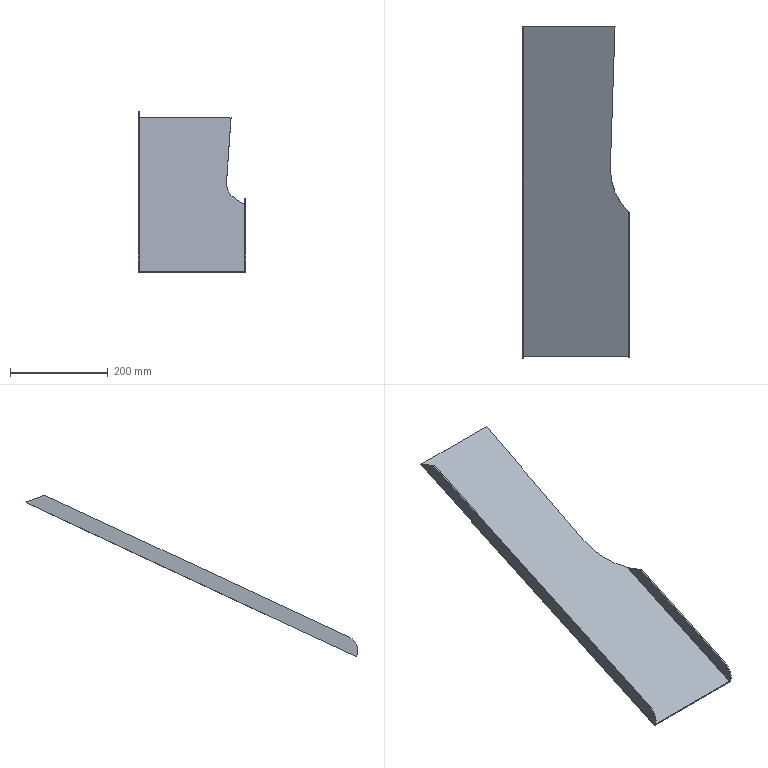Part | NX | features solid 2 | 1 solid | 15 faces | box 219.206 x 677.811 x 330.114 mm | volume 356857 mm3 | plane 12 | cylinder 2 | spline 1 | commonest cylinder face diameters 60 x2
STEP:
#1=CARTESIAN_POINT('',(-1052.794,-840.,-504.758));
#2=VERTEX_POINT('',#1);
#3=CARTESIAN_POINT('',(-1268.,-840.,-504.758));
#4=VERTEX_POINT('',#3);
#5=CARTESIAN_POINT('',(-476.248,-840.,-504.758));
#6=DIRECTION('',(1.,0.,0.));
#7=VECTOR('',#6,1000.);
#8=LINE('',#5,#7);
#9=EDGE_CURVE('',#2,#4,#8,.F.);
#10=ORIENTED_EDGE('',*,*,#9,.F.);
#11=CARTESIAN_POINT('',(-1052.794,-840.,-502.551));
#12=VERTEX_POINT('',#11);
#13=CARTESIAN_POINT('',(-1052.794,-840.,-720.));
#14=DIRECTION('',(0.,0.,-1.));
#15=VECTOR('',#14,1000.);
#16=LINE('',#13,#15);
#17=EDGE_CURVE('',#2,#12,#16,.F.);
#18=ORIENTED_EDGE('',*,*,#17,.T.);
#19=CARTESIAN_POINT('',(-1268.,-840.,-502.551));
#20=VERTEX_POINT('',#19);
#21=CARTESIAN_POINT('',(-476.248,-840.,-502.551));
#22=DIRECTION('',(1.,0.,0.));
#23=VECTOR('',#22,1000.);
#24=LINE('',#21,#23);
#25=EDGE_CURVE('',#12,#20,#24,.F.);
#26=ORIENTED_EDGE('',*,*,#25,.T.);
#27=CARTESIAN_POINT('',(-1268.,-840.,-720.));
#28=DIRECTION('',(0.,0.,1.));
#29=VECTOR('',#28,1000.);
#30=LINE('',#27,#29);
#31=EDGE_CURVE('',#20,#4,#30,.F.);
#32=ORIENTED_EDGE('',*,*,#31,.T.);
#33=EDGE_LOOP('',(#10,#18,#26,#32));
#34=FACE_BOUND('',#33,.T.);
#35=CARTESIAN_POINT('',(-476.248,-840.,-720.));
#36=DIRECTION('',(0.,1.,0.));
#37=DIRECTION('',(-1.,0.,0.));
#38=AXIS2_PLACEMENT_3D('',#35,#36,#37);
#39=PLANE('',#38);
#40=ADVANCED_FACE('',(#34),#39,.F.);
#41=ORIENTED_EDGE('',*,*,#25,.F.);
#42=CARTESIAN_POINT('',(-1052.794,-547.056,-365.949));
#43=VERTEX_POINT('',#42);
#44=CARTESIAN_POINT('',(-1052.794,-618.999,-399.497));
#45=DIRECTION('',(0.,0.9063,0.4226));
#46=VECTOR('',#45,1000.);
#47=LINE('',#44,#46);
#48=EDGE_CURVE('',#12,#43,#47,.T.);
#49=ORIENTED_EDGE('',*,*,#48,.T.);
#50=CARTESIAN_POINT('',(-1050.794,-547.056,-365.949));
#51=VERTEX_POINT('',#50);
#52=CARTESIAN_POINT('',(-1050.794,-547.056,-365.949));
#53=DIRECTION('',(-1.,0.,0.));
#54=VECTOR('',#53,1000.);
#55=LINE('',#52,#54);
#56=EDGE_CURVE('',#43,#51,#55,.F.);
#57=ORIENTED_EDGE('',*,*,#56,.T.);
#58=CARTESIAN_POINT('',(-1080.711,-165.845,-188.187));
#59=VERTEX_POINT('',#58);
#60=CARTESIAN_POINT('',(-1050.794,-547.056,-365.949));
#61=CARTESIAN_POINT('',(-1053.882,-544.25,-364.64));
#62=CARTESIAN_POINT('',(-1058.306,-539.762,-362.548));
#63=CARTESIAN_POINT('',(-1063.751,-533.278,-359.524));
#64=CARTESIAN_POINT('',(-1067.683,-528.054,-357.088));
#65=CARTESIAN_POINT('',(-1071.168,-522.909,-354.689));
#66=CARTESIAN_POINT('',(-1075.487,-515.815,-351.381));
#67=CARTESIAN_POINT('',(-1080.162,-506.646,-347.106));
#68=CARTESIAN_POINT('',(-1083.845,-497.104,-342.656));
#69=CARTESIAN_POINT('',(-1086.159,-489.295,-339.014));
#70=CARTESIAN_POINT('',(-1087.595,-483.291,-336.215));
#71=CARTESIAN_POINT('',(-1088.504,-478.353,-333.912));
#72=CARTESIAN_POINT('',(-1089.084,-474.355,-332.048));
#73=CARTESIAN_POINT('',(-1089.448,-471.284,-330.616));
#74=CARTESIAN_POINT('',(-1089.716,-468.409,-329.275));
#75=CARTESIAN_POINT('',(-1089.93,-465.381,-327.863));
#76=CARTESIAN_POINT('',(-1090.054,-462.819,-326.669));
#77=CARTESIAN_POINT('',(-1090.114,-460.972,-325.807));
#78=CARTESIAN_POINT('',(-1090.14,-459.934,-325.323));
#79=CARTESIAN_POINT('',(-1090.157,-459.074,-324.922));
#80=CARTESIAN_POINT('',(-1090.165,-458.504,-324.657));
#81=CARTESIAN_POINT('',(-1090.174,-457.614,-324.242));
#82=CARTESIAN_POINT('',(-1090.181,-456.046,-323.51));
#83=CARTESIAN_POINT('',(-1090.168,-454.094,-322.6));
#84=CARTESIAN_POINT('',(-1090.134,-452.013,-321.63));
#85=CARTESIAN_POINT('',(-1090.097,-450.378,-320.867));
#86=CARTESIAN_POINT('',(-1090.059,-448.97,-320.211));
#87=CARTESIAN_POINT('',(-1090.026,-447.93,-319.725));
#88=CARTESIAN_POINT('',(-1090.008,-447.366,-319.463));
#89=CARTESIAN_POINT('',(-1089.989,-446.827,-319.211));
#90=CARTESIAN_POINT('',(-1089.985,-446.712,-319.158));
#91=CARTESIAN_POINT('',(-1089.973,-446.372,-318.999));
#92=CARTESIAN_POINT('',(-1089.951,-445.769,-318.718));
#93=CARTESIAN_POINT('',(-1089.909,-444.636,-318.19));
#94=CARTESIAN_POINT('',(-1089.854,-443.221,-317.53));
#95=CARTESIAN_POINT('',(-1089.809,-442.047,-316.982));
#96=CARTESIAN_POINT('',(-1089.782,-441.361,-316.663));
#97=CARTESIAN_POINT('',(-1089.757,-440.736,-316.371));
#98=CARTESIAN_POINT('',(-1089.745,-440.425,-316.226));
#99=CARTESIAN_POINT('',(-1089.725,-439.901,-315.981));
#100=CARTESIAN_POINT('',(-1089.691,-439.031,-315.576));
#101=CARTESIAN_POINT('',(-1089.642,-437.754,-314.98));
#102=CARTESIAN_POINT('',(-1089.595,-436.484,-314.388));
#103=CARTESIAN_POINT('',(-1089.562,-435.575,-313.965));
#104=CARTESIAN_POINT('',(-1089.544,-435.076,-313.732));
#105=CARTESIAN_POINT('',(-1089.528,-434.64,-313.528));
#106=CARTESIAN_POINT('',(-1089.521,-434.438,-313.434));
#107=CARTESIAN_POINT('',(-1089.508,-434.08,-313.267));
#108=CARTESIAN_POINT('',(-1089.486,-433.479,-312.987));
#109=CARTESIAN_POINT('',(-1089.454,-432.557,-312.557));
#110=CARTESIAN_POINT('',(-1089.414,-431.394,-312.015));
#111=CARTESIAN_POINT('',(-1089.358,-429.753,-311.25));
#112=CARTESIAN_POINT('',(-1089.284,-427.537,-310.216));
#113=CARTESIAN_POINT('',(-1089.188,-424.614,-308.853));
#114=CARTESIAN_POINT('',(-1089.086,-421.427,-307.367));
#115=CARTESIAN_POINT('',(-1088.996,-418.551,-306.026));
#116=CARTESIAN_POINT('',(-1088.92,-416.12,-304.892));
#117=CARTESIAN_POINT('',(-1088.861,-414.227,-304.01));
#118=CARTESIAN_POINT('',(-1088.811,-412.603,-303.252));
#119=CARTESIAN_POINT('',(-1088.775,-411.422,-302.702));
#120=CARTESIAN_POINT('',(-1088.755,-410.763,-302.394));
#121=CARTESIAN_POINT('',(-1088.737,-410.198,-302.131));
#122=CARTESIAN_POINT('',(-1088.728,-409.88,-301.983));
#123=CARTESIAN_POINT('',(-1088.712,-409.369,-301.745));
#124=CARTESIAN_POINT('',(-1088.686,-408.516,-301.346));
#125=CARTESIAN_POINT('',(-1088.648,-407.273,-300.767));
#126=CARTESIAN_POINT('',(-1088.602,-405.788,-300.074));
#127=CARTESIAN_POINT('',(-1088.541,-403.8,-299.148));
#128=CARTESIAN_POINT('',(-1088.463,-401.309,-297.986));
#129=CARTESIAN_POINT('',(-1088.338,-397.307,-296.12));
#130=CARTESIAN_POINT('',(-1088.179,-392.276,-293.774));
#131=CARTESIAN_POINT('',(-1087.919,-384.16,-289.989));
#132=CARTESIAN_POINT('',(-1087.584,-373.902,-285.206));
#133=CARTESIAN_POINT('',(-1087.163,-361.377,-279.365));
#134=CARTESIAN_POINT('',(-1086.735,-348.748,-273.476));
#135=CARTESIAN_POINT('',(-1086.316,-336.279,-267.662));
#136=CARTESIAN_POINT('',(-1085.901,-323.9,-261.889));
#137=CARTESIAN_POINT('',(-1085.492,-311.629,-256.167));
#138=CARTESIAN_POINT('',(-1085.156,-301.489,-251.439));
#139=CARTESIAN_POINT('',(-1084.89,-293.43,-247.681));
#140=CARTESIAN_POINT('',(-1084.691,-287.411,-244.875));
#141=CARTESIAN_POINT('',(-1084.494,-281.419,-242.08));
#142=CARTESIAN_POINT('',(-1084.331,-276.447,-239.762));
#143=CARTESIAN_POINT('',(-1084.202,-272.483,-237.913));
#144=CARTESIAN_POINT('',(-1084.121,-270.011,-236.761));
#145=CARTESIAN_POINT('',(-1084.056,-268.035,-235.839));
#146=CARTESIAN_POINT('',(-1084.008,-266.558,-235.151));
#147=CARTESIAN_POINT('',(-1083.968,-265.32,-234.573));
#148=CARTESIAN_POINT('',(-1083.94,-264.472,-234.178));
#149=CARTESIAN_POINT('',(-1083.923,-263.958,-233.938));
#150=CARTESIAN_POINT('',(-1083.914,-263.655,-233.797));
#151=CARTESIAN_POINT('',(-1083.894,-263.041,-233.511));
#152=CARTESIAN_POINT('',(-1083.871,-262.333,-233.18));
#153=CARTESIAN_POINT('',(-1083.829,-261.048,-232.581));
#154=CARTESIAN_POINT('',(-1083.77,-259.252,-231.744));
#155=CARTESIAN_POINT('',(-1083.7,-257.106,-230.743));
#156=CARTESIAN_POINT('',(-1083.608,-254.277,-229.424));
#157=CARTESIAN_POINT('',(-1083.494,-250.791,-227.798));
#158=CARTESIAN_POINT('',(-1083.316,-245.326,-225.25));
#159=CARTESIAN_POINT('',(-1083.1,-238.703,-222.162));
#160=CARTESIAN_POINT('',(-1082.852,-231.09,-218.612));
#161=CARTESIAN_POINT('',(-1082.614,-223.811,-215.217));
#162=CARTESIAN_POINT('',(-1082.312,-214.551,-210.899));
#163=CARTESIAN_POINT('',(-1081.96,-203.811,-205.891));
#164=CARTESIAN_POINT('',(-1081.582,-192.259,-200.504));
#165=CARTESIAN_POINT('',(-1081.134,-178.639,-194.153));
#166=CARTESIAN_POINT('',(-1080.863,-170.428,-190.324));
#167=CARTESIAN_POINT('',(-1080.711,-165.845,-188.187));
#168=B_SPLINE_CURVE_WITH_KNOTS('',3,(#60,#61,#62,#63,#64,#65,#66,#67,#68,#69,#70,#71,#72,#73,#74,#75,#76,#77,#78,#79,#80,#81,#82,#83,#84,#85,#86,#87,#88,#89,#90,#91,#92,#93,#94,#95,#96,#97,#98,#99,#100,#101,#102,#103,#104,#105,#106,#107,#108,#109,#110,#111,#112,#113,#114,#115,#116,#117,#118,#119,#120,#121,#122,#123,#124,#125,#126,#127,#128,#129,#130,#131,#132,#133,#134,#135,#136,#137,#138,#139,#140,#141,#142,#143,#144,#145,#146,#147,#148,#149,#150,#151,#152,#153,#154,#155,#156,#157,#158,#159,#160,#161,#162,#163,#164,#165,#166,#167),.UNSPECIFIED.,.F.,.F.,(4,1,1,1,1,1,1,1,1,1,1,1,1,1,1,1,1,1,1,1,1,1,1,1,1,1,1,1,1,1,1,1,1,1,1,1,1,1,1,1,1,1,1,1,1,1,1,1,1,1,1,1,1,1,1,1,1,1,1,1,1,1,1,1,1,1,1,1,1,1,1,1,1,1,1,1,1,1,1,1,1,1,1,1,1,1,1,1,1,1,1,1,1,1,1,1,1,1,1,1,1,1,1,1,1,4),(0.,0.03125,0.04688,0.0625,0.07812,0.09375,0.125,0.1562,0.1719,0.1875,0.2031,0.2109,0.2188,0.2266,0.2344,0.2422,0.2461,0.248,0.25,0.252,0.2539,0.2578,0.2656,0.2695,0.2734,0.2773,0.2793,0.2803,0.2812,0.2822,0.2832,0.2852,0.2891,0.293,0.2949,0.2959,0.2969,0.2979,0.2988,0.3008,0.3047,0.3086,0.3105,0.3115,0.3125,0.3135,0.3145,0.3164,0.3203,0.3242,0.3281,0.3359,0.3438,0.3516,0.3594,0.3633,0.3672,0.3711,0.373,0.374,0.375,0.376,0.377,0.3789,0.3828,0.3867,0.3906,0.3984,0.4062,0.4219,0.4375,0.4688,0.5,0.5312,0.5625,0.5938,0.625,0.6562,0.6719,0.6875,0.7031,0.7188,0.7266,0.7344,0.7383,0.7422,0.7461,0.748,0.749,0.75,0.751,0.752,0.7539,0.7578,0.7617,0.7656,0.7734,0.7812,0.7969,0.8125,0.8281,0.8438,0.875,0.9062,0.9375,1.),.UNSPECIFIED.);
#169=EDGE_CURVE('',#59,#51,#168,.F.);
#170=ORIENTED_EDGE('',*,*,#169,.F.);
#171=CARTESIAN_POINT('',(-1268.,-165.845,-188.187));
#172=VERTEX_POINT('',#171);
#173=CARTESIAN_POINT('',(-1078.278,-165.845,-188.187));
#174=DIRECTION('',(1.,0.,0.));
#175=VECTOR('',#174,1000.);
#176=LINE('',#173,#175);
#177=EDGE_CURVE('',#172,#59,#176,.T.);
#178=ORIENTED_EDGE('',*,*,#177,.F.);
#179=CARTESIAN_POINT('',(-1268.,-618.999,-399.497));
#180=DIRECTION('',(0.,-0.9063,-0.4226));
#181=VECTOR('',#180,1000.);
#182=LINE('',#179,#181);
#183=EDGE_CURVE('',#172,#20,#182,.T.);
#184=ORIENTED_EDGE('',*,*,#183,.T.);
#185=EDGE_LOOP('',(#41,#49,#57,#170,#178,#184));
#186=FACE_BOUND('',#185,.T.);
#187=CARTESIAN_POINT('',(-1078.278,-618.999,-399.497));
#188=DIRECTION('',(0.,-0.4226,0.9063));
#189=DIRECTION('',(1.,0.,0.));
#190=AXIS2_PLACEMENT_3D('',#187,#188,#189);
#191=PLANE('',#190);
#192=ADVANCED_FACE('',(#186),#191,.T.);
#193=CARTESIAN_POINT('',(-1270.,-165.,-190.));
#194=VERTEX_POINT('',#193);
#195=CARTESIAN_POINT('',(-1270.,-840.,-504.758));
#196=VERTEX_POINT('',#195);
#197=CARTESIAN_POINT('',(-1270.,619.132,175.647));
#198=DIRECTION('',(0.,-0.9063,-0.4226));
#199=VECTOR('',#198,1000.);
#200=LINE('',#197,#199);
#201=EDGE_CURVE('',#194,#196,#200,.T.);
#202=ORIENTED_EDGE('',*,*,#201,.T.);
#203=CARTESIAN_POINT('',(-1270.,-825.489,-464.89));
#204=VERTEX_POINT('',#203);
#205=CARTESIAN_POINT('',(-1270.,-812.811,-492.079));
#206=DIRECTION('',(-1.,0.,0.));
#207=DIRECTION('',(0.,0.,1.));
#208=AXIS2_PLACEMENT_3D('',#205,#206,#207);
#209=CIRCLE('',#208,30.);
#210=EDGE_CURVE('',#196,#204,#209,.T.);
#211=ORIENTED_EDGE('',*,*,#210,.T.);
#212=CARTESIAN_POINT('',(-1270.,-203.055,-174.644));
#213=VERTEX_POINT('',#212);
#214=CARTESIAN_POINT('',(-1270.,-177.679,-162.811));
#215=DIRECTION('',(0.,-0.9063,-0.4226));
#216=VECTOR('',#215,1000.);
#217=LINE('',#214,#216);
#218=EDGE_CURVE('',#213,#204,#217,.T.);
#219=ORIENTED_EDGE('',*,*,#218,.F.);
#220=CARTESIAN_POINT('',(-1270.,-165.845,-188.187));
#221=VERTEX_POINT('',#220);
#222=CARTESIAN_POINT('',(-1270.,-164.516,-188.671));
#223=DIRECTION('',(0.,-0.9397,0.342));
#224=VECTOR('',#223,1000.);
#225=LINE('',#222,#224);
#226=EDGE_CURVE('',#213,#221,#225,.F.);
#227=ORIENTED_EDGE('',*,*,#226,.T.);
#228=CARTESIAN_POINT('',(-1270.,-165.845,-188.187));
#229=DIRECTION('',(0.,0.4226,-0.9063));
#230=VECTOR('',#229,1000.);
#231=LINE('',#228,#230);
#232=EDGE_CURVE('',#221,#194,#231,.T.);
#233=ORIENTED_EDGE('',*,*,#232,.T.);
#234=EDGE_LOOP('',(#202,#211,#219,#227,#233));
#235=FACE_BOUND('',#234,.T.);
#236=CARTESIAN_POINT('',(-1270.,618.287,177.459));
#237=DIRECTION('',(1.,0.,0.));
#238=DIRECTION('',(0.,0.,-1.));
#239=AXIS2_PLACEMENT_3D('',#236,#237,#238);
#240=PLANE('',#239);
#241=ADVANCED_FACE('',(#235),#240,.F.);
#242=CARTESIAN_POINT('',(-1050.794,-825.489,-464.89));
#243=VERTEX_POINT('',#242);
#244=CARTESIAN_POINT('',(-1050.794,-840.,-504.758));
#245=VERTEX_POINT('',#244);
#246=CARTESIAN_POINT('',(-1050.794,-812.811,-492.079));
#247=DIRECTION('',(1.,0.,0.));
#248=DIRECTION('',(0.,0.,-1.));
#249=AXIS2_PLACEMENT_3D('',#246,#247,#248);
#250=CIRCLE('',#249,30.);
#251=EDGE_CURVE('',#243,#245,#250,.T.);
#252=ORIENTED_EDGE('',*,*,#251,.T.);
#253=CARTESIAN_POINT('',(-1050.794,-546.211,-367.761));
#254=VERTEX_POINT('',#253);
#255=CARTESIAN_POINT('',(-1050.794,-618.154,-401.309));
#256=DIRECTION('',(0.,0.9063,0.4226));
#257=VECTOR('',#256,1000.);
#258=LINE('',#255,#257);
#259=EDGE_CURVE('',#245,#254,#258,.T.);
#260=ORIENTED_EDGE('',*,*,#259,.T.);
#261=CARTESIAN_POINT('',(-1050.794,-546.211,-367.761));
#262=CARTESIAN_POINT('',(-1050.794,-546.492,-367.157));
#263=CARTESIAN_POINT('',(-1050.794,-546.774,-366.553));
#264=CARTESIAN_POINT('',(-1050.794,-547.056,-365.949));
#265=B_SPLINE_CURVE_WITH_KNOTS('',3,(#261,#262,#263,#264),.UNSPECIFIED.,.F.,.F.,(4,4),(0.,1.),.UNSPECIFIED.);
#266=EDGE_CURVE('',#51,#254,#265,.F.);
#267=ORIENTED_EDGE('',*,*,#266,.F.);
#268=CARTESIAN_POINT('',(-1050.794,-584.266,-352.406));
#269=VERTEX_POINT('',#268);
#270=CARTESIAN_POINT('',(-1050.794,-761.12,-288.036));
#271=DIRECTION('',(0.,-0.9397,0.342));
#272=VECTOR('',#271,1000.);
#273=LINE('',#270,#272);
#274=EDGE_CURVE('',#51,#269,#273,.T.);
#275=ORIENTED_EDGE('',*,*,#274,.T.);
#276=CARTESIAN_POINT('',(-1050.794,-852.679,-477.568));
#277=DIRECTION('',(0.,0.9063,0.4226));
#278=VECTOR('',#277,1000.);
#279=LINE('',#276,#278);
#280=EDGE_CURVE('',#243,#269,#279,.T.);
#281=ORIENTED_EDGE('',*,*,#280,.F.);
#282=EDGE_LOOP('',(#252,#260,#267,#275,#281));
#283=FACE_BOUND('',#282,.T.);
#284=CARTESIAN_POINT('',(-1050.794,-618.999,-399.497));
#285=DIRECTION('',(-1.,0.,0.));
#286=DIRECTION('',(0.,0.,1.));
#287=AXIS2_PLACEMENT_3D('',#284,#285,#286);
#288=PLANE('',#287);
#289=ADVANCED_FACE('',(#283),#288,.F.);
#290=CARTESIAN_POINT('',(-1080.711,-165.,-190.));
#291=VERTEX_POINT('',#290);
#292=CARTESIAN_POINT('',(-1050.794,-546.211,-367.761));
#293=CARTESIAN_POINT('',(-1053.882,-543.405,-366.453));
#294=CARTESIAN_POINT('',(-1058.306,-538.917,-364.36));
#295=CARTESIAN_POINT('',(-1063.751,-532.433,-361.337));
#296=CARTESIAN_POINT('',(-1067.683,-527.209,-358.901));
#297=CARTESIAN_POINT('',(-1071.168,-522.064,-356.502));
#298=CARTESIAN_POINT('',(-1075.487,-514.969,-353.193));
#299=CARTESIAN_POINT('',(-1080.162,-505.801,-348.918));
#300=CARTESIAN_POINT('',(-1083.845,-496.258,-344.468));
#301=CARTESIAN_POINT('',(-1086.159,-488.449,-340.827));
#302=CARTESIAN_POINT('',(-1087.595,-482.446,-338.027));
#303=CARTESIAN_POINT('',(-1088.504,-477.508,-335.725));
#304=CARTESIAN_POINT('',(-1089.084,-473.51,-333.86));
#305=CARTESIAN_POINT('',(-1089.448,-470.439,-332.428));
#306=CARTESIAN_POINT('',(-1089.716,-467.563,-331.088));
#307=CARTESIAN_POINT('',(-1089.93,-464.535,-329.676));
#308=CARTESIAN_POINT('',(-1090.054,-461.974,-328.481));
#309=CARTESIAN_POINT('',(-1090.114,-460.126,-327.62));
#310=CARTESIAN_POINT('',(-1090.14,-459.089,-327.136));
#311=CARTESIAN_POINT('',(-1090.157,-458.229,-326.735));
#312=CARTESIAN_POINT('',(-1090.165,-457.659,-326.469));
#313=CARTESIAN_POINT('',(-1090.174,-456.769,-326.054));
#314=CARTESIAN_POINT('',(-1090.181,-455.201,-325.323));
#315=CARTESIAN_POINT('',(-1090.168,-453.249,-324.413));
#316=CARTESIAN_POINT('',(-1090.134,-451.168,-323.442));
#317=CARTESIAN_POINT('',(-1090.097,-449.532,-322.68));
#318=CARTESIAN_POINT('',(-1090.059,-448.125,-322.023));
#319=CARTESIAN_POINT('',(-1090.026,-447.084,-321.538));
#320=CARTESIAN_POINT('',(-1090.008,-446.521,-321.275));
#321=CARTESIAN_POINT('',(-1089.989,-445.982,-321.024));
#322=CARTESIAN_POINT('',(-1089.985,-445.866,-320.97));
#323=CARTESIAN_POINT('',(-1089.973,-445.526,-320.812));
#324=CARTESIAN_POINT('',(-1089.951,-444.923,-320.53));
#325=CARTESIAN_POINT('',(-1089.909,-443.791,-320.002));
#326=CARTESIAN_POINT('',(-1089.854,-442.376,-319.343));
#327=CARTESIAN_POINT('',(-1089.809,-441.202,-318.795));
#328=CARTESIAN_POINT('',(-1089.782,-440.516,-318.475));
#329=CARTESIAN_POINT('',(-1089.757,-439.89,-318.184));
#330=CARTESIAN_POINT('',(-1089.745,-439.58,-318.039));
#331=CARTESIAN_POINT('',(-1089.725,-439.055,-317.794));
#332=CARTESIAN_POINT('',(-1089.691,-438.186,-317.389));
#333=CARTESIAN_POINT('',(-1089.642,-436.908,-316.793));
#334=CARTESIAN_POINT('',(-1089.595,-435.639,-316.201));
#335=CARTESIAN_POINT('',(-1089.562,-434.73,-315.777));
#336=CARTESIAN_POINT('',(-1089.544,-434.231,-315.545));
#337=CARTESIAN_POINT('',(-1089.528,-433.795,-315.341));
#338=CARTESIAN_POINT('',(-1089.521,-433.593,-315.247));
#339=CARTESIAN_POINT('',(-1089.508,-433.235,-315.08));
#340=CARTESIAN_POINT('',(-1089.486,-432.633,-314.799));
#341=CARTESIAN_POINT('',(-1089.454,-431.712,-314.37));
#342=CARTESIAN_POINT('',(-1089.414,-430.549,-313.828));
#343=CARTESIAN_POINT('',(-1089.358,-428.908,-313.062));
#344=CARTESIAN_POINT('',(-1089.284,-426.692,-312.029));
#345=CARTESIAN_POINT('',(-1089.188,-423.769,-310.666));
#346=CARTESIAN_POINT('',(-1089.086,-420.582,-309.18));
#347=CARTESIAN_POINT('',(-1088.996,-417.706,-307.839));
#348=CARTESIAN_POINT('',(-1088.92,-415.274,-306.705));
#349=CARTESIAN_POINT('',(-1088.861,-413.382,-305.822));
#350=CARTESIAN_POINT('',(-1088.811,-411.758,-305.065));
#351=CARTESIAN_POINT('',(-1088.775,-410.577,-304.514));
#352=CARTESIAN_POINT('',(-1088.755,-409.917,-304.207));
#353=CARTESIAN_POINT('',(-1088.737,-409.353,-303.944));
#354=CARTESIAN_POINT('',(-1088.728,-409.035,-303.795));
#355=CARTESIAN_POINT('',(-1088.712,-408.524,-303.557));
#356=CARTESIAN_POINT('',(-1088.686,-407.67,-303.159));
#357=CARTESIAN_POINT('',(-1088.648,-406.428,-302.58));
#358=CARTESIAN_POINT('',(-1088.602,-404.942,-301.887));
#359=CARTESIAN_POINT('',(-1088.541,-402.955,-300.96));
#360=CARTESIAN_POINT('',(-1088.463,-400.464,-299.799));
#361=CARTESIAN_POINT('',(-1088.338,-396.462,-297.933));
#362=CARTESIAN_POINT('',(-1088.179,-391.431,-295.586));
#363=CARTESIAN_POINT('',(-1087.919,-383.315,-291.802));
#364=CARTESIAN_POINT('',(-1087.584,-373.057,-287.018));
#365=CARTESIAN_POINT('',(-1087.163,-360.532,-281.178));
#366=CARTESIAN_POINT('',(-1086.735,-347.903,-275.289));
#367=CARTESIAN_POINT('',(-1086.316,-335.434,-269.475));
#368=CARTESIAN_POINT('',(-1085.901,-323.054,-263.702));
#369=CARTESIAN_POINT('',(-1085.492,-310.783,-257.98));
#370=CARTESIAN_POINT('',(-1085.156,-300.644,-253.252));
#371=CARTESIAN_POINT('',(-1084.89,-292.584,-249.494));
#372=CARTESIAN_POINT('',(-1084.691,-286.566,-246.687));
#373=CARTESIAN_POINT('',(-1084.494,-280.574,-243.893));
#374=CARTESIAN_POINT('',(-1084.331,-275.602,-241.575));
#375=CARTESIAN_POINT('',(-1084.202,-271.637,-239.726));
#376=CARTESIAN_POINT('',(-1084.121,-269.165,-238.573));
#377=CARTESIAN_POINT('',(-1084.056,-267.19,-237.652));
#378=CARTESIAN_POINT('',(-1084.008,-265.713,-236.963));
#379=CARTESIAN_POINT('',(-1083.968,-264.474,-236.386));
#380=CARTESIAN_POINT('',(-1083.94,-263.626,-235.99));
#381=CARTESIAN_POINT('',(-1083.923,-263.113,-235.751));
#382=CARTESIAN_POINT('',(-1083.914,-262.81,-235.609));
#383=CARTESIAN_POINT('',(-1083.894,-262.196,-235.323));
#384=CARTESIAN_POINT('',(-1083.871,-261.488,-234.993));
#385=CARTESIAN_POINT('',(-1083.829,-260.203,-234.394));
#386=CARTESIAN_POINT('',(-1083.77,-258.407,-233.556));
#387=CARTESIAN_POINT('',(-1083.7,-256.261,-232.556));
#388=CARTESIAN_POINT('',(-1083.608,-253.432,-231.236));
#389=CARTESIAN_POINT('',(-1083.494,-249.946,-229.611));
#390=CARTESIAN_POINT('',(-1083.316,-244.481,-227.063));
#391=CARTESIAN_POINT('',(-1083.1,-237.858,-223.974));
#392=CARTESIAN_POINT('',(-1082.852,-230.245,-220.424));
#393=CARTESIAN_POINT('',(-1082.614,-222.966,-217.03));
#394=CARTESIAN_POINT('',(-1082.312,-213.706,-212.712));
#395=CARTESIAN_POINT('',(-1081.96,-202.966,-207.704));
#396=CARTESIAN_POINT('',(-1081.582,-191.414,-202.317));
#397=CARTESIAN_POINT('',(-1081.134,-177.794,-195.966));
#398=CARTESIAN_POINT('',(-1080.863,-169.583,-192.137));
#399=CARTESIAN_POINT('',(-1080.711,-165.,-190.));
#400=B_SPLINE_CURVE_WITH_KNOTS('',3,(#292,#293,#294,#295,#296,#297,#298,#299,#300,#301,#302,#303,#304,#305,#306,#307,#308,#309,#310,#311,#312,#313,#314,#315,#316,#317,#318,#319,#320,#321,#322,#323,#324,#325,#326,#327,#328,#329,#330,#331,#332,#333,#334,#335,#336,#337,#338,#339,#340,#341,#342,#343,#344,#345,#346,#347,#348,#349,#350,#351,#352,#353,#354,#355,#356,#357,#358,#359,#360,#361,#362,#363,#364,#365,#366,#367,#368,#369,#370,#371,#372,#373,#374,#375,#376,#377,#378,#379,#380,#381,#382,#383,#384,#385,#386,#387,#388,#389,#390,#391,#392,#393,#394,#395,#396,#397,#398,#399),.UNSPECIFIED.,.F.,.F.,(4,1,1,1,1,1,1,1,1,1,1,1,1,1,1,1,1,1,1,1,1,1,1,1,1,1,1,1,1,1,1,1,1,1,1,1,1,1,1,1,1,1,1,1,1,1,1,1,1,1,1,1,1,1,1,1,1,1,1,1,1,1,1,1,1,1,1,1,1,1,1,1,1,1,1,1,1,1,1,1,1,1,1,1,1,1,1,1,1,1,1,1,1,1,1,1,1,1,1,1,1,1,1,1,1,4),(0.,0.03125,0.04688,0.0625,0.07812,0.09375,0.125,0.1562,0.1719,0.1875,0.2031,0.2109,0.2188,0.2266,0.2344,0.2422,0.2461,0.248,0.25,0.252,0.2539,0.2578,0.2656,0.2695,0.2734,0.2773,0.2793,0.2803,0.2812,0.2822,0.2832,0.2852,0.2891,0.293,0.2949,0.2959,0.2969,0.2979,0.2988,0.3008,0.3047,0.3086,0.3105,0.3115,0.3125,0.3135,0.3145,0.3164,0.3203,0.3242,0.3281,0.3359,0.3438,0.3516,0.3594,0.3633,0.3672,0.3711,0.373,0.374,0.375,0.376,0.377,0.3789,0.3828,0.3867,0.3906,0.3984,0.4062,0.4219,0.4375,0.4688,0.5,0.5312,0.5625,0.5938,0.625,0.6562,0.6719,0.6875,0.7031,0.7188,0.7266,0.7344,0.7383,0.7422,0.7461,0.748,0.749,0.75,0.751,0.752,0.7539,0.7578,0.7617,0.7656,0.7734,0.7812,0.7969,0.8125,0.8281,0.8438,0.875,0.9062,0.9375,1.),.UNSPECIFIED.);
#401=EDGE_CURVE('',#291,#254,#400,.F.);
#402=ORIENTED_EDGE('',*,*,#401,.F.);
#403=CARTESIAN_POINT('',(-1080.711,-165.845,-188.187));
#404=CARTESIAN_POINT('',(-1080.711,-165.563,-188.792));
#405=CARTESIAN_POINT('',(-1080.711,-165.282,-189.396));
#406=CARTESIAN_POINT('',(-1080.711,-165.,-190.));
#407=B_SPLINE_CURVE_WITH_KNOTS('',3,(#403,#404,#405,#406),.UNSPECIFIED.,.F.,.F.,(4,4),(0.,1.),.UNSPECIFIED.);
#408=EDGE_CURVE('',#59,#291,#407,.T.);
#409=ORIENTED_EDGE('',*,*,#408,.F.);
#410=ORIENTED_EDGE('',*,*,#169,.T.);
#411=ORIENTED_EDGE('',*,*,#266,.T.);
#412=EDGE_LOOP('',(#402,#409,#410,#411));
#413=FACE_BOUND('',#412,.T.);
#414=CARTESIAN_POINT('',(-1050.794,-547.056,-365.949));
#415=CARTESIAN_POINT('',(-1050.794,-546.211,-367.761));
#416=CARTESIAN_POINT('',(-1053.882,-544.25,-364.64));
#417=CARTESIAN_POINT('',(-1053.882,-543.405,-366.453));
#418=CARTESIAN_POINT('',(-1058.306,-539.762,-362.548));
#419=CARTESIAN_POINT('',(-1058.306,-538.917,-364.36));
#420=CARTESIAN_POINT('',(-1063.751,-533.278,-359.524));
#421=CARTESIAN_POINT('',(-1063.751,-532.433,-361.337));
#422=CARTESIAN_POINT('',(-1067.683,-528.054,-357.088));
#423=CARTESIAN_POINT('',(-1067.683,-527.209,-358.901));
#424=CARTESIAN_POINT('',(-1071.168,-522.909,-354.689));
#425=CARTESIAN_POINT('',(-1071.168,-522.064,-356.502));
#426=CARTESIAN_POINT('',(-1075.487,-515.815,-351.381));
#427=CARTESIAN_POINT('',(-1075.487,-514.969,-353.193));
#428=CARTESIAN_POINT('',(-1080.162,-506.646,-347.106));
#429=CARTESIAN_POINT('',(-1080.162,-505.801,-348.918));
#430=CARTESIAN_POINT('',(-1083.845,-497.104,-342.656));
#431=CARTESIAN_POINT('',(-1083.845,-496.258,-344.468));
#432=CARTESIAN_POINT('',(-1086.159,-489.295,-339.014));
#433=CARTESIAN_POINT('',(-1086.159,-488.449,-340.827));
#434=CARTESIAN_POINT('',(-1087.595,-483.291,-336.215));
#435=CARTESIAN_POINT('',(-1087.595,-482.446,-338.027));
#436=CARTESIAN_POINT('',(-1088.504,-478.353,-333.912));
#437=CARTESIAN_POINT('',(-1088.504,-477.508,-335.725));
#438=CARTESIAN_POINT('',(-1089.084,-474.355,-332.048));
#439=CARTESIAN_POINT('',(-1089.084,-473.51,-333.86));
#440=CARTESIAN_POINT('',(-1089.448,-471.284,-330.616));
#441=CARTESIAN_POINT('',(-1089.448,-470.439,-332.428));
#442=CARTESIAN_POINT('',(-1089.716,-468.409,-329.275));
#443=CARTESIAN_POINT('',(-1089.716,-467.563,-331.088));
#444=CARTESIAN_POINT('',(-1089.93,-465.381,-327.863));
#445=CARTESIAN_POINT('',(-1089.93,-464.535,-329.676));
#446=CARTESIAN_POINT('',(-1090.054,-462.819,-326.669));
#447=CARTESIAN_POINT('',(-1090.054,-461.974,-328.481));
#448=CARTESIAN_POINT('',(-1090.114,-460.972,-325.807));
#449=CARTESIAN_POINT('',(-1090.114,-460.126,-327.62));
#450=CARTESIAN_POINT('',(-1090.14,-459.934,-325.323));
#451=CARTESIAN_POINT('',(-1090.14,-459.089,-327.136));
#452=CARTESIAN_POINT('',(-1090.157,-459.074,-324.922));
#453=CARTESIAN_POINT('',(-1090.157,-458.229,-326.735));
#454=CARTESIAN_POINT('',(-1090.165,-458.504,-324.657));
#455=CARTESIAN_POINT('',(-1090.165,-457.659,-326.469));
#456=CARTESIAN_POINT('',(-1090.174,-457.614,-324.242));
#457=CARTESIAN_POINT('',(-1090.174,-456.769,-326.054));
#458=CARTESIAN_POINT('',(-1090.181,-456.046,-323.51));
#459=CARTESIAN_POINT('',(-1090.181,-455.201,-325.323));
#460=CARTESIAN_POINT('',(-1090.168,-454.094,-322.6));
#461=CARTESIAN_POINT('',(-1090.168,-453.249,-324.413));
#462=CARTESIAN_POINT('',(-1090.134,-452.013,-321.63));
#463=CARTESIAN_POINT('',(-1090.134,-451.168,-323.442));
#464=CARTESIAN_POINT('',(-1090.097,-450.378,-320.867));
#465=CARTESIAN_POINT('',(-1090.097,-449.532,-322.68));
#466=CARTESIAN_POINT('',(-1090.059,-448.97,-320.211));
#467=CARTESIAN_POINT('',(-1090.059,-448.125,-322.023));
#468=CARTESIAN_POINT('',(-1090.026,-447.93,-319.725));
#469=CARTESIAN_POINT('',(-1090.026,-447.084,-321.538));
#470=CARTESIAN_POINT('',(-1090.008,-447.366,-319.463));
#471=CARTESIAN_POINT('',(-1090.008,-446.521,-321.275));
#472=CARTESIAN_POINT('',(-1089.989,-446.827,-319.211));
#473=CARTESIAN_POINT('',(-1089.989,-445.982,-321.024));
#474=CARTESIAN_POINT('',(-1089.985,-446.712,-319.158));
#475=CARTESIAN_POINT('',(-1089.985,-445.866,-320.97));
#476=CARTESIAN_POINT('',(-1089.973,-446.372,-318.999));
#477=CARTESIAN_POINT('',(-1089.973,-445.526,-320.812));
#478=CARTESIAN_POINT('',(-1089.951,-445.769,-318.718));
#479=CARTESIAN_POINT('',(-1089.951,-444.923,-320.53));
#480=CARTESIAN_POINT('',(-1089.909,-444.636,-318.19));
#481=CARTESIAN_POINT('',(-1089.909,-443.791,-320.002));
#482=CARTESIAN_POINT('',(-1089.854,-443.221,-317.53));
#483=CARTESIAN_POINT('',(-1089.854,-442.376,-319.343));
#484=CARTESIAN_POINT('',(-1089.809,-442.047,-316.982));
#485=CARTESIAN_POINT('',(-1089.809,-441.202,-318.795));
#486=CARTESIAN_POINT('',(-1089.782,-441.361,-316.663));
#487=CARTESIAN_POINT('',(-1089.782,-440.516,-318.475));
#488=CARTESIAN_POINT('',(-1089.757,-440.736,-316.371));
#489=CARTESIAN_POINT('',(-1089.757,-439.89,-318.184));
#490=CARTESIAN_POINT('',(-1089.745,-440.425,-316.226));
#491=CARTESIAN_POINT('',(-1089.745,-439.58,-318.039));
#492=CARTESIAN_POINT('',(-1089.725,-439.901,-315.981));
#493=CARTESIAN_POINT('',(-1089.725,-439.055,-317.794));
#494=CARTESIAN_POINT('',(-1089.691,-439.031,-315.576));
#495=CARTESIAN_POINT('',(-1089.691,-438.186,-317.389));
#496=CARTESIAN_POINT('',(-1089.642,-437.754,-314.98));
#497=CARTESIAN_POINT('',(-1089.642,-436.908,-316.793));
#498=CARTESIAN_POINT('',(-1089.595,-436.484,-314.388));
#499=CARTESIAN_POINT('',(-1089.595,-435.639,-316.201));
#500=CARTESIAN_POINT('',(-1089.562,-435.575,-313.965));
#501=CARTESIAN_POINT('',(-1089.562,-434.73,-315.777));
#502=CARTESIAN_POINT('',(-1089.544,-435.076,-313.732));
#503=CARTESIAN_POINT('',(-1089.544,-434.231,-315.545));
#504=CARTESIAN_POINT('',(-1089.528,-434.64,-313.528));
#505=CARTESIAN_POINT('',(-1089.528,-433.795,-315.341));
#506=CARTESIAN_POINT('',(-1089.521,-434.438,-313.434));
#507=CARTESIAN_POINT('',(-1089.521,-433.593,-315.247));
#508=CARTESIAN_POINT('',(-1089.508,-434.08,-313.267));
#509=CARTESIAN_POINT('',(-1089.508,-433.235,-315.08));
#510=CARTESIAN_POINT('',(-1089.486,-433.479,-312.987));
#511=CARTESIAN_POINT('',(-1089.486,-432.633,-314.799));
#512=CARTESIAN_POINT('',(-1089.454,-432.557,-312.557));
#513=CARTESIAN_POINT('',(-1089.454,-431.712,-314.37));
#514=CARTESIAN_POINT('',(-1089.414,-431.394,-312.015));
#515=CARTESIAN_POINT('',(-1089.414,-430.549,-313.828));
#516=CARTESIAN_POINT('',(-1089.358,-429.753,-311.25));
#517=CARTESIAN_POINT('',(-1089.358,-428.908,-313.062));
#518=CARTESIAN_POINT('',(-1089.284,-427.537,-310.216));
#519=CARTESIAN_POINT('',(-1089.284,-426.692,-312.029));
#520=CARTESIAN_POINT('',(-1089.188,-424.614,-308.853));
#521=CARTESIAN_POINT('',(-1089.188,-423.769,-310.666));
#522=CARTESIAN_POINT('',(-1089.086,-421.427,-307.367));
#523=CARTESIAN_POINT('',(-1089.086,-420.582,-309.18));
#524=CARTESIAN_POINT('',(-1088.996,-418.551,-306.026));
#525=CARTESIAN_POINT('',(-1088.996,-417.706,-307.839));
#526=CARTESIAN_POINT('',(-1088.92,-416.12,-304.892));
#527=CARTESIAN_POINT('',(-1088.92,-415.274,-306.705));
#528=CARTESIAN_POINT('',(-1088.861,-414.227,-304.01));
#529=CARTESIAN_POINT('',(-1088.861,-413.382,-305.822));
#530=CARTESIAN_POINT('',(-1088.811,-412.603,-303.252));
#531=CARTESIAN_POINT('',(-1088.811,-411.758,-305.065));
#532=CARTESIAN_POINT('',(-1088.775,-411.422,-302.702));
#533=CARTESIAN_POINT('',(-1088.775,-410.577,-304.514));
#534=CARTESIAN_POINT('',(-1088.755,-410.763,-302.394));
#535=CARTESIAN_POINT('',(-1088.755,-409.917,-304.207));
#536=CARTESIAN_POINT('',(-1088.737,-410.198,-302.131));
#537=CARTESIAN_POINT('',(-1088.737,-409.353,-303.944));
#538=CARTESIAN_POINT('',(-1088.728,-409.88,-301.983));
#539=CARTESIAN_POINT('',(-1088.728,-409.035,-303.795));
#540=CARTESIAN_POINT('',(-1088.712,-409.369,-301.745));
#541=CARTESIAN_POINT('',(-1088.712,-408.524,-303.557));
#542=CARTESIAN_POINT('',(-1088.686,-408.516,-301.346));
#543=CARTESIAN_POINT('',(-1088.686,-407.67,-303.159));
#544=CARTESIAN_POINT('',(-1088.648,-407.273,-300.767));
#545=CARTESIAN_POINT('',(-1088.648,-406.428,-302.58));
#546=CARTESIAN_POINT('',(-1088.602,-405.788,-300.074));
#547=CARTESIAN_POINT('',(-1088.602,-404.942,-301.887));
#548=CARTESIAN_POINT('',(-1088.541,-403.8,-299.148));
#549=CARTESIAN_POINT('',(-1088.541,-402.955,-300.96));
#550=CARTESIAN_POINT('',(-1088.463,-401.309,-297.986));
#551=CARTESIAN_POINT('',(-1088.463,-400.464,-299.799));
#552=CARTESIAN_POINT('',(-1088.338,-397.307,-296.12));
#553=CARTESIAN_POINT('',(-1088.338,-396.462,-297.933));
#554=CARTESIAN_POINT('',(-1088.179,-392.276,-293.774));
#555=CARTESIAN_POINT('',(-1088.179,-391.431,-295.586));
#556=CARTESIAN_POINT('',(-1087.919,-384.16,-289.989));
#557=CARTESIAN_POINT('',(-1087.919,-383.315,-291.802));
#558=CARTESIAN_POINT('',(-1087.584,-373.902,-285.206));
#559=CARTESIAN_POINT('',(-1087.584,-373.057,-287.018));
#560=CARTESIAN_POINT('',(-1087.163,-361.377,-279.365));
#561=CARTESIAN_POINT('',(-1087.163,-360.532,-281.178));
#562=CARTESIAN_POINT('',(-1086.735,-348.748,-273.476));
#563=CARTESIAN_POINT('',(-1086.735,-347.903,-275.289));
#564=CARTESIAN_POINT('',(-1086.316,-336.279,-267.662));
#565=CARTESIAN_POINT('',(-1086.316,-335.434,-269.475));
#566=CARTESIAN_POINT('',(-1085.901,-323.9,-261.889));
#567=CARTESIAN_POINT('',(-1085.901,-323.054,-263.702));
#568=CARTESIAN_POINT('',(-1085.492,-311.629,-256.167));
#569=CARTESIAN_POINT('',(-1085.492,-310.783,-257.98));
#570=CARTESIAN_POINT('',(-1085.156,-301.489,-251.439));
#571=CARTESIAN_POINT('',(-1085.156,-300.644,-253.252));
#572=CARTESIAN_POINT('',(-1084.89,-293.43,-247.681));
#573=CARTESIAN_POINT('',(-1084.89,-292.584,-249.494));
#574=CARTESIAN_POINT('',(-1084.691,-287.411,-244.875));
#575=CARTESIAN_POINT('',(-1084.691,-286.566,-246.687));
#576=CARTESIAN_POINT('',(-1084.494,-281.419,-242.08));
#577=CARTESIAN_POINT('',(-1084.494,-280.574,-243.893));
#578=CARTESIAN_POINT('',(-1084.331,-276.447,-239.762));
#579=CARTESIAN_POINT('',(-1084.331,-275.602,-241.575));
#580=CARTESIAN_POINT('',(-1084.202,-272.483,-237.913));
#581=CARTESIAN_POINT('',(-1084.202,-271.637,-239.726));
#582=CARTESIAN_POINT('',(-1084.121,-270.011,-236.761));
#583=CARTESIAN_POINT('',(-1084.121,-269.165,-238.573));
#584=CARTESIAN_POINT('',(-1084.056,-268.035,-235.839));
#585=CARTESIAN_POINT('',(-1084.056,-267.19,-237.652));
#586=CARTESIAN_POINT('',(-1084.008,-266.558,-235.151));
#587=CARTESIAN_POINT('',(-1084.008,-265.713,-236.963));
#588=CARTESIAN_POINT('',(-1083.968,-265.32,-234.573));
#589=CARTESIAN_POINT('',(-1083.968,-264.474,-236.386));
#590=CARTESIAN_POINT('',(-1083.94,-264.472,-234.178));
#591=CARTESIAN_POINT('',(-1083.94,-263.626,-235.99));
#592=CARTESIAN_POINT('',(-1083.923,-263.958,-233.938));
#593=CARTESIAN_POINT('',(-1083.923,-263.113,-235.751));
#594=CARTESIAN_POINT('',(-1083.914,-263.655,-233.797));
#595=CARTESIAN_POINT('',(-1083.914,-262.81,-235.609));
#596=CARTESIAN_POINT('',(-1083.894,-263.041,-233.511));
#597=CARTESIAN_POINT('',(-1083.894,-262.196,-235.323));
#598=CARTESIAN_POINT('',(-1083.871,-262.333,-233.18));
#599=CARTESIAN_POINT('',(-1083.871,-261.488,-234.993));
#600=CARTESIAN_POINT('',(-1083.829,-261.048,-232.581));
#601=CARTESIAN_POINT('',(-1083.829,-260.203,-234.394));
#602=CARTESIAN_POINT('',(-1083.77,-259.252,-231.744));
#603=CARTESIAN_POINT('',(-1083.77,-258.407,-233.556));
#604=CARTESIAN_POINT('',(-1083.7,-257.106,-230.743));
#605=CARTESIAN_POINT('',(-1083.7,-256.261,-232.556));
#606=CARTESIAN_POINT('',(-1083.608,-254.277,-229.424));
#607=CARTESIAN_POINT('',(-1083.608,-253.432,-231.236));
#608=CARTESIAN_POINT('',(-1083.494,-250.791,-227.798));
#609=CARTESIAN_POINT('',(-1083.494,-249.946,-229.611));
#610=CARTESIAN_POINT('',(-1083.316,-245.326,-225.25));
#611=CARTESIAN_POINT('',(-1083.316,-244.481,-227.063));
#612=CARTESIAN_POINT('',(-1083.1,-238.703,-222.162));
#613=CARTESIAN_POINT('',(-1083.1,-237.858,-223.974));
#614=CARTESIAN_POINT('',(-1082.852,-231.09,-218.612));
#615=CARTESIAN_POINT('',(-1082.852,-230.245,-220.424));
#616=CARTESIAN_POINT('',(-1082.614,-223.811,-215.217));
#617=CARTESIAN_POINT('',(-1082.614,-222.966,-217.03));
#618=CARTESIAN_POINT('',(-1081.706,-196.031,-202.263));
#619=CARTESIAN_POINT('',(-1081.706,-195.185,-204.076));
#620=CARTESIAN_POINT('',(-1081.091,-177.303,-193.53));
#621=CARTESIAN_POINT('',(-1081.091,-176.457,-195.343));
#622=CARTESIAN_POINT('',(-1080.711,-165.845,-188.187));
#623=CARTESIAN_POINT('',(-1080.711,-165.,-190.));
#624=B_SPLINE_SURFACE_WITH_KNOTS('',3,1,((#414,#415),(#416,#417),(#418,#419),(#420,#421),(#422,#423),(#424,#425),(#426,#427),(#428,#429),(#430,#431),(#432,#433),(#434,#435),(#436,#437),(#438,#439),(#440,#441),(#442,#443),(#444,#445),(#446,#447),(#448,#449),(#450,#451),(#452,#453),(#454,#455),(#456,#457),(#458,#459),(#460,#461),(#462,#463),(#464,#465),(#466,#467),(#468,#469),(#470,#471),(#472,#473),(#474,#475),(#476,#477),(#478,#479),(#480,#481),(#482,#483),(#484,#485),(#486,#487),(#488,#489),(#490,#491),(#492,#493),(#494,#495),(#496,#497),(#498,#499),(#500,#501),(#502,#503),(#504,#505),(#506,#507),(#508,#509),(#510,#511),(#512,#513),(#514,#515),(#516,#517),(#518,#519),(#520,#521),(#522,#523),(#524,#525),(#526,#527),(#528,#529),(#530,#531),(#532,#533),(#534,#535),(#536,#537),(#538,#539),(#540,#541),(#542,#543),(#544,#545),(#546,#547),(#548,#549),(#550,#551),(#552,#553),(#554,#555),(#556,#557),(#558,#559),(#560,#561),(#562,#563),(#564,#565),(#566,#567),(#568,#569),(#570,#571),(#572,#573),(#574,#575),(#576,#577),(#578,#579),(#580,#581),(#582,#583),(#584,#585),(#586,#587),(#588,#589),(#590,#591),(#592,#593),(#594,#595),(#596,#597),(#598,#599),(#600,#601),(#602,#603),(#604,#605),(#606,#607),(#608,#609),(#610,#611),(#612,#613),(#614,#615),(#616,#617),(#618,#619),(#620,#621),(#622,#623)),.UNSPECIFIED.,.F.,.F.,.F.,(4,1,1,1,1,1,1,1,1,1,1,1,1,1,1,1,1,1,1,1,1,1,1,1,1,1,1,1,1,1,1,1,1,1,1,1,1,1,1,1,1,1,1,1,1,1,1,1,1,1,1,1,1,1,1,1,1,1,1,1,1,1,1,1,1,1,1,1,1,1,1,1,1,1,1,1,1,1,1,1,1,1,1,1,1,1,1,1,1,1,1,1,1,1,1,1,1,1,1,1,1,1,4),(2,2),(0.,0.03125,0.04688,0.0625,0.07812,0.09375,0.125,0.1562,0.1719,0.1875,0.2031,0.2109,0.2188,0.2266,0.2344,0.2422,0.2461,0.248,0.25,0.252,0.2539,0.2578,0.2656,0.2695,0.2734,0.2773,0.2793,0.2803,0.2812,0.2822,0.2832,0.2852,0.2891,0.293,0.2949,0.2959,0.2969,0.2979,0.2988,0.3008,0.3047,0.3086,0.3105,0.3115,0.3125,0.3135,0.3145,0.3164,0.3203,0.3242,0.3281,0.3359,0.3438,0.3516,0.3594,0.3633,0.3672,0.3711,0.373,0.374,0.375,0.376,0.377,0.3789,0.3828,0.3867,0.3906,0.3984,0.4062,0.4219,0.4375,0.4688,0.5,0.5312,0.5625,0.5938,0.625,0.6562,0.6719,0.6875,0.7031,0.7188,0.7266,0.7344,0.7383,0.7422,0.7461,0.748,0.749,0.75,0.751,0.752,0.7539,0.7578,0.7617,0.7656,0.7734,0.7812,0.7969,0.8125,0.8281,0.8438,1.),(0.,1.),.UNSPECIFIED.);
#625=ADVANCED_FACE('',(#413),#624,.F.);
#626=CARTESIAN_POINT('',(-1078.278,-165.845,-188.187));
#627=DIRECTION('',(1.,0.,0.));
#628=VECTOR('',#627,1000.);
#629=LINE('',#626,#628);
#630=EDGE_CURVE('',#221,#172,#629,.T.);
#631=ORIENTED_EDGE('',*,*,#630,.T.);
#632=ORIENTED_EDGE('',*,*,#177,.T.);
#633=ORIENTED_EDGE('',*,*,#408,.T.);
#634=CARTESIAN_POINT('',(-1078.278,-165.,-190.));
#635=DIRECTION('',(1.,0.,0.));
#636=VECTOR('',#635,1000.);
#637=LINE('',#634,#636);
#638=EDGE_CURVE('',#194,#291,#637,.T.);
#639=ORIENTED_EDGE('',*,*,#638,.F.);
#640=ORIENTED_EDGE('',*,*,#232,.F.);
#641=EDGE_LOOP('',(#631,#632,#633,#639,#640));
#642=FACE_BOUND('',#641,.T.);
#643=CARTESIAN_POINT('',(-1078.278,-165.845,-188.187));
#644=DIRECTION('',(0.,0.9063,0.4226));
#645=DIRECTION('',(0.,-0.4226,0.9063));
#646=AXIS2_PLACEMENT_3D('',#643,#644,#645);
#647=PLANE('',#646);
#648=ADVANCED_FACE('',(#642),#647,.T.);
#649=ORIENTED_EDGE('',*,*,#401,.T.);
#650=ORIENTED_EDGE('',*,*,#259,.F.);
#651=CARTESIAN_POINT('',(-476.248,-840.,-504.758));
#652=DIRECTION('',(1.,0.,0.));
#653=VECTOR('',#652,1000.);
#654=LINE('',#651,#653);
#655=EDGE_CURVE('',#245,#2,#654,.F.);
#656=ORIENTED_EDGE('',*,*,#655,.T.);
#657=ORIENTED_EDGE('',*,*,#9,.T.);
#658=CARTESIAN_POINT('',(-1270.,-840.,-504.758));
#659=DIRECTION('',(1.,0.,0.));
#660=VECTOR('',#659,1000.);
#661=LINE('',#658,#660);
#662=EDGE_CURVE('',#196,#4,#661,.T.);
#663=ORIENTED_EDGE('',*,*,#662,.F.);
#664=ORIENTED_EDGE('',*,*,#201,.F.);
#665=ORIENTED_EDGE('',*,*,#638,.T.);
#666=EDGE_LOOP('',(#649,#650,#656,#657,#663,#664,#665));
#667=FACE_BOUND('',#666,.T.);
#668=CARTESIAN_POINT('',(-1078.278,-618.154,-401.309));
#669=DIRECTION('',(0.,-0.4226,0.9063));
#670=DIRECTION('',(1.,0.,0.));
#671=AXIS2_PLACEMENT_3D('',#668,#669,#670);
#672=PLANE('',#671);
#673=ADVANCED_FACE('',(#667),#672,.F.);
#674=ORIENTED_EDGE('',*,*,#218,.T.);
#675=CARTESIAN_POINT('',(-1268.,-825.489,-464.89));
#676=VERTEX_POINT('',#675);
#677=CARTESIAN_POINT('',(-1270.,-825.489,-464.89));
#678=DIRECTION('',(1.,0.,0.));
#679=VECTOR('',#678,1000.);
#680=LINE('',#677,#679);
#681=EDGE_CURVE('',#204,#676,#680,.T.);
#682=ORIENTED_EDGE('',*,*,#681,.T.);
#683=CARTESIAN_POINT('',(-1268.,-203.055,-174.644));
#684=VERTEX_POINT('',#683);
#685=CARTESIAN_POINT('',(-1268.,-177.679,-162.811));
#686=DIRECTION('',(0.,-0.9063,-0.4226));
#687=VECTOR('',#686,1000.);
#688=LINE('',#685,#687);
#689=EDGE_CURVE('',#684,#676,#688,.T.);
#690=ORIENTED_EDGE('',*,*,#689,.F.);
#691=CARTESIAN_POINT('',(-1270.,-203.055,-174.644));
#692=DIRECTION('',(1.,0.,0.));
#693=VECTOR('',#692,1000.);
#694=LINE('',#691,#693);
#695=EDGE_CURVE('',#684,#213,#694,.F.);
#696=ORIENTED_EDGE('',*,*,#695,.T.);
#697=EDGE_LOOP('',(#674,#682,#690,#696));
#698=FACE_BOUND('',#697,.T.);
#699=CARTESIAN_POINT('',(-1270.,-177.679,-162.811));
#700=DIRECTION('',(0.,0.4226,-0.9063));
#701=DIRECTION('',(0.,-0.9063,-0.4226));
#702=AXIS2_PLACEMENT_3D('',#699,#700,#701);
#703=PLANE('',#702);
#704=ADVANCED_FACE('',(#698),#703,.F.);
#705=ORIENTED_EDGE('',*,*,#31,.F.);
#706=ORIENTED_EDGE('',*,*,#183,.F.);
#707=CARTESIAN_POINT('',(-1268.,-165.845,-188.187));
#708=DIRECTION('',(0.,0.9397,-0.342));
#709=VECTOR('',#708,1000.);
#710=LINE('',#707,#709);
#711=EDGE_CURVE('',#172,#684,#710,.F.);
#712=ORIENTED_EDGE('',*,*,#711,.T.);
#713=ORIENTED_EDGE('',*,*,#689,.T.);
#714=CARTESIAN_POINT('',(-1268.,-812.811,-492.079));
#715=DIRECTION('',(-1.,0.,0.));
#716=DIRECTION('',(0.,0.,1.));
#717=AXIS2_PLACEMENT_3D('',#714,#715,#716);
#718=CIRCLE('',#717,30.);
#719=EDGE_CURVE('',#676,#4,#718,.F.);
#720=ORIENTED_EDGE('',*,*,#719,.T.);
#721=EDGE_LOOP('',(#705,#706,#712,#713,#720));
#722=FACE_BOUND('',#721,.T.);
#723=CARTESIAN_POINT('',(-1268.,-165.,-190.));
#724=DIRECTION('',(-1.,0.,0.));
#725=DIRECTION('',(0.,0.,1.));
#726=AXIS2_PLACEMENT_3D('',#723,#724,#725);
#727=PLANE('',#726);
#728=ADVANCED_FACE('',(#722),#727,.F.);
#729=ORIENTED_EDGE('',*,*,#226,.F.);
#730=ORIENTED_EDGE('',*,*,#695,.F.);
#731=ORIENTED_EDGE('',*,*,#711,.F.);
#732=ORIENTED_EDGE('',*,*,#630,.F.);
#733=EDGE_LOOP('',(#729,#730,#731,#732));
#734=FACE_BOUND('',#733,.T.);
#735=CARTESIAN_POINT('',(-1270.,-165.845,-188.187));
#736=DIRECTION('',(0.,-0.342,-0.9397));
#737=DIRECTION('',(0.,0.9397,-0.342));
#738=AXIS2_PLACEMENT_3D('',#735,#736,#737);
#739=PLANE('',#738);
#740=ADVANCED_FACE('',(#734),#739,.F.);
#741=ORIENTED_EDGE('',*,*,#210,.F.);
#742=ORIENTED_EDGE('',*,*,#662,.T.);
#743=ORIENTED_EDGE('',*,*,#719,.F.);
#744=ORIENTED_EDGE('',*,*,#681,.F.);
#745=EDGE_LOOP('',(#741,#742,#743,#744));
#746=FACE_BOUND('',#745,.T.);
#747=CARTESIAN_POINT('',(-1270.,-812.811,-492.079));
#748=DIRECTION('',(-1.,0.,0.));
#749=DIRECTION('',(0.,0.,1.));
#750=AXIS2_PLACEMENT_3D('',#747,#748,#749);
#751=CYLINDRICAL_SURFACE('',#750,30.);
#752=ADVANCED_FACE('',(#746),#751,.T.);
#753=CARTESIAN_POINT('',(-1052.794,-825.489,-464.89));
#754=VERTEX_POINT('',#753);
#755=CARTESIAN_POINT('',(-1052.794,-584.266,-352.406));
#756=VERTEX_POINT('',#755);
#757=CARTESIAN_POINT('',(-1052.794,-852.679,-477.568));
#758=DIRECTION('',(0.,0.9063,0.4226));
#759=VECTOR('',#758,1000.);
#760=LINE('',#757,#759);
#761=EDGE_CURVE('',#754,#756,#760,.T.);
#762=ORIENTED_EDGE('',*,*,#761,.F.);
#763=CARTESIAN_POINT('',(-1050.794,-825.489,-464.89));
#764=DIRECTION('',(-1.,0.,0.));
#765=VECTOR('',#764,1000.);
#766=LINE('',#763,#765);
#767=EDGE_CURVE('',#754,#243,#766,.F.);
#768=ORIENTED_EDGE('',*,*,#767,.T.);
#769=ORIENTED_EDGE('',*,*,#280,.T.);
#770=CARTESIAN_POINT('',(-1050.794,-584.266,-352.406));
#771=DIRECTION('',(-1.,0.,0.));
#772=VECTOR('',#771,1000.);
#773=LINE('',#770,#772);
#774=EDGE_CURVE('',#269,#756,#773,.T.);
#775=ORIENTED_EDGE('',*,*,#774,.T.);
#776=EDGE_LOOP('',(#762,#768,#769,#775));
#777=FACE_BOUND('',#776,.T.);
#778=CARTESIAN_POINT('',(-1050.794,-852.679,-477.568));
#779=DIRECTION('',(0.,0.4226,-0.9063));
#780=DIRECTION('',(0.,0.9063,0.4226));
#781=AXIS2_PLACEMENT_3D('',#778,#779,#780);
#782=PLANE('',#781);
#783=ADVANCED_FACE('',(#777),#782,.F.);
#784=ORIENTED_EDGE('',*,*,#17,.F.);
#785=CARTESIAN_POINT('',(-1052.794,-812.811,-492.079));
#786=DIRECTION('',(1.,0.,0.));
#787=DIRECTION('',(0.,0.,-1.));
#788=AXIS2_PLACEMENT_3D('',#785,#786,#787);
#789=CIRCLE('',#788,30.);
#790=EDGE_CURVE('',#2,#754,#789,.F.);
#791=ORIENTED_EDGE('',*,*,#790,.T.);
#792=ORIENTED_EDGE('',*,*,#761,.T.);
#793=CARTESIAN_POINT('',(-1052.794,-584.266,-352.406));
#794=DIRECTION('',(0.,0.9397,-0.342));
#795=VECTOR('',#794,1000.);
#796=LINE('',#793,#795);
#797=EDGE_CURVE('',#756,#43,#796,.T.);
#798=ORIENTED_EDGE('',*,*,#797,.T.);
#799=ORIENTED_EDGE('',*,*,#48,.F.);
#800=EDGE_LOOP('',(#784,#791,#792,#798,#799));
#801=FACE_BOUND('',#800,.T.);
#802=CARTESIAN_POINT('',(-1052.794,-840.,-504.758));
#803=DIRECTION('',(1.,0.,0.));
#804=DIRECTION('',(0.,0.,-1.));
#805=AXIS2_PLACEMENT_3D('',#802,#803,#804);
#806=PLANE('',#805);
#807=ADVANCED_FACE('',(#801),#806,.F.);
#808=ORIENTED_EDGE('',*,*,#274,.F.);
#809=ORIENTED_EDGE('',*,*,#56,.F.);
#810=ORIENTED_EDGE('',*,*,#797,.F.);
#811=ORIENTED_EDGE('',*,*,#774,.F.);
#812=EDGE_LOOP('',(#808,#809,#810,#811));
#813=FACE_BOUND('',#812,.T.);
#814=CARTESIAN_POINT('',(-1050.794,-584.266,-352.406));
#815=DIRECTION('',(0.,0.342,0.9397));
#816=DIRECTION('',(0.,-0.9397,0.342));
#817=AXIS2_PLACEMENT_3D('',#814,#815,#816);
#818=PLANE('',#817);
#819=ADVANCED_FACE('',(#813),#818,.T.);
#820=ORIENTED_EDGE('',*,*,#251,.F.);
#821=ORIENTED_EDGE('',*,*,#767,.F.);
#822=ORIENTED_EDGE('',*,*,#790,.F.);
#823=ORIENTED_EDGE('',*,*,#655,.F.);
#824=EDGE_LOOP('',(#820,#821,#822,#823));
#825=FACE_BOUND('',#824,.T.);
#826=CARTESIAN_POINT('',(-1050.794,-812.811,-492.079));
#827=DIRECTION('',(-1.,0.,0.));
#828=DIRECTION('',(0.,0.,1.));
#829=AXIS2_PLACEMENT_3D('',#826,#827,#828);
#830=CYLINDRICAL_SURFACE('',#829,30.);
#831=ADVANCED_FACE('',(#825),#830,.T.);
#832=CLOSED_SHELL('',(#40,#192,#241,#289,#625,#648,#673,#704,#728,#740,#752,#783,#807,#819,#831));
#833=MANIFOLD_SOLID_BREP('',#832);
#834=(LENGTH_UNIT()NAMED_UNIT(*)SI_UNIT(.MILLI.,.METRE.));
#835=UNCERTAINTY_MEASURE_WITH_UNIT(LENGTH_MEASURE(0.0508),#834,'','');
#836=(NAMED_UNIT(*)PLANE_ANGLE_UNIT()SI_UNIT($,.RADIAN.));
#837=(NAMED_UNIT(*)SI_UNIT($,.STERADIAN.)SOLID_ANGLE_UNIT());
#838=(GEOMETRIC_REPRESENTATION_CONTEXT(3)GLOBAL_UNCERTAINTY_ASSIGNED_CONTEXT((#835))GLOBAL_UNIT_ASSIGNED_CONTEXT((#834,#836,#837))REPRESENTATION_CONTEXT('',''));
#839=ADVANCED_BREP_SHAPE_REPRESENTATION('',(#833),#838);